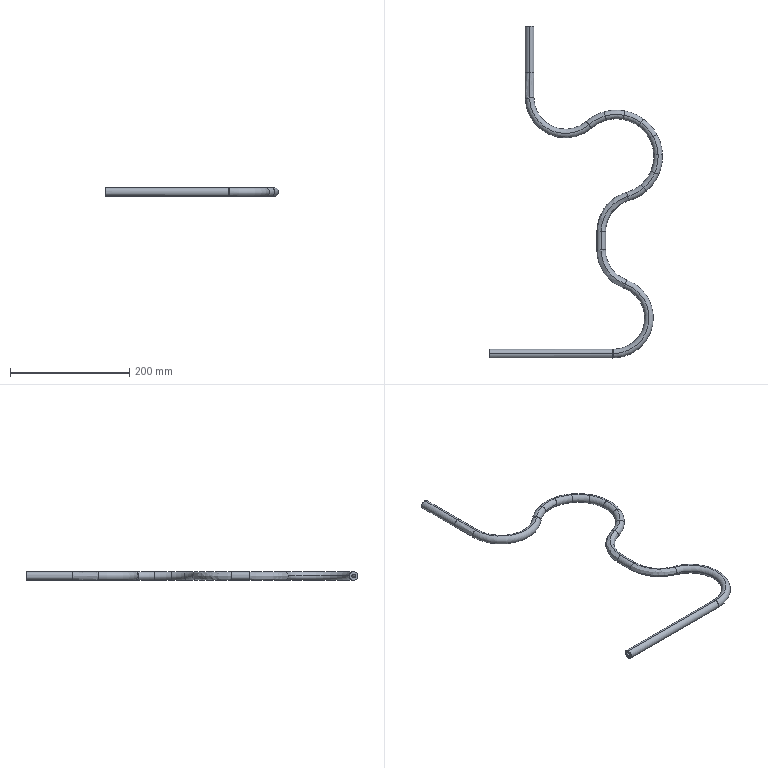Part | NX | features BREP 1 | 1 solid | 79 faces | box 289.488 x 555.807 x 14.5 mm | volume 142372 mm3 | torus 41 | cylinder 22 | spline 14 | plane 2 | commonest cylinder face diameters 6.35 x12 14.5 x10